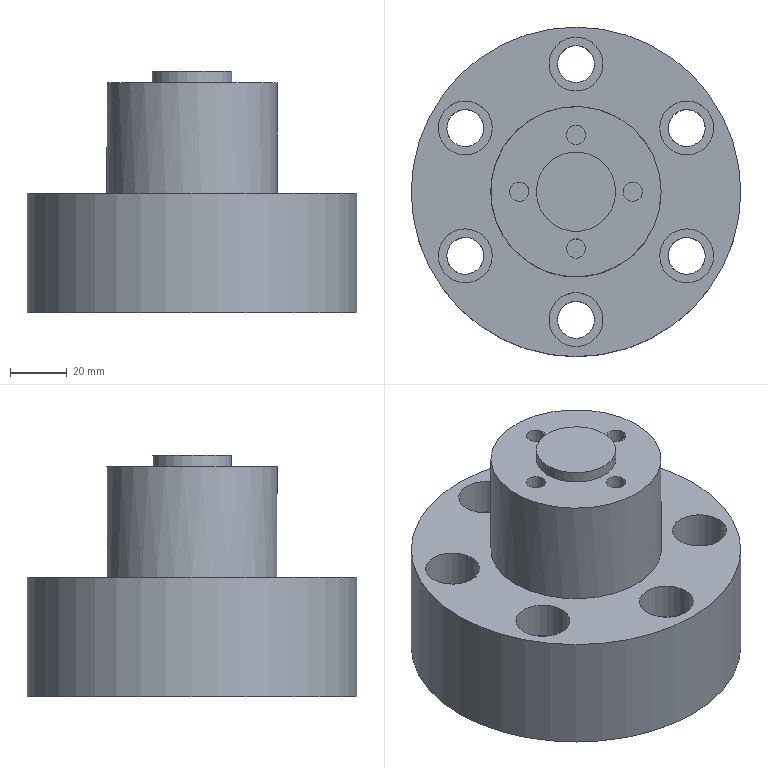Part | NX | 1 solid | 33 faces | box 116 x 116 x 85 mm | volume 509067 mm3 | cylinder 19 | plane 14 | commonest cylinder face diameters 13 x6 19 x6 6.8 x4 28 x1 60 x1 116 x1
STEP:
#1=CARTESIAN_POINT('',(-42.221,16.871,-85.));
#2=VERTEX_POINT('',#1);
#3=CARTESIAN_POINT('',(-38.971,22.5,-85.));
#4=DIRECTION('',(0.,0.,1.));
#5=DIRECTION('',(-0.5,-0.866,0.));
#6=AXIS2_PLACEMENT_3D('',#3,#4,#5);
#7=CIRCLE('',#6,6.5);
#8=EDGE_CURVE('',#2,#2,#7,.T.);
#9=ORIENTED_EDGE('',*,*,#8,.F.);
#10=EDGE_LOOP('',(#9));
#11=FACE_BOUND('',#10,.T.);
#12=CARTESIAN_POINT('',(-32.471,22.5,-56.));
#13=VERTEX_POINT('',#12);
#14=CARTESIAN_POINT('',(-38.971,22.5,-56.));
#15=DIRECTION('',(0.,0.,1.));
#16=DIRECTION('',(1.,0.,0.));
#17=AXIS2_PLACEMENT_3D('',#14,#15,#16);
#18=CIRCLE('',#17,6.5);
#19=EDGE_CURVE('',#13,#13,#18,.F.);
#20=ORIENTED_EDGE('',*,*,#19,.F.);
#21=EDGE_LOOP('',(#20));
#22=FACE_BOUND('',#21,.T.);
#23=CARTESIAN_POINT('',(-38.971,22.5,-85.));
#24=DIRECTION('',(0.,0.,1.));
#25=DIRECTION('',(1.,0.,0.));
#26=AXIS2_PLACEMENT_3D('',#23,#24,#25);
#27=CYLINDRICAL_SURFACE('',#26,6.5);
#28=ADVANCED_FACE('',(#11,#22),#27,.F.);
#29=CARTESIAN_POINT('',(6.5,-45.,-85.));
#30=VERTEX_POINT('',#29);
#31=CARTESIAN_POINT('',(0.,-45.,-85.));
#32=DIRECTION('',(0.,0.,1.));
#33=DIRECTION('',(1.,0.,0.));
#34=AXIS2_PLACEMENT_3D('',#31,#32,#33);
#35=CIRCLE('',#34,6.5);
#36=EDGE_CURVE('',#30,#30,#35,.T.);
#37=ORIENTED_EDGE('',*,*,#36,.F.);
#38=EDGE_LOOP('',(#37));
#39=FACE_BOUND('',#38,.T.);
#40=CARTESIAN_POINT('',(6.5,-45.,-56.));
#41=VERTEX_POINT('',#40);
#42=CARTESIAN_POINT('',(0.,-45.,-56.));
#43=DIRECTION('',(0.,0.,1.));
#44=DIRECTION('',(1.,0.,0.));
#45=AXIS2_PLACEMENT_3D('',#42,#43,#44);
#46=CIRCLE('',#45,6.5);
#47=EDGE_CURVE('',#41,#41,#46,.F.);
#48=ORIENTED_EDGE('',*,*,#47,.F.);
#49=EDGE_LOOP('',(#48));
#50=FACE_BOUND('',#49,.T.);
#51=CARTESIAN_POINT('',(0.,-45.,-85.));
#52=DIRECTION('',(0.,0.,1.));
#53=DIRECTION('',(1.,0.,0.));
#54=AXIS2_PLACEMENT_3D('',#51,#52,#53);
#55=CYLINDRICAL_SURFACE('',#54,6.5);
#56=ADVANCED_FACE('',(#39,#50),#55,.F.);
#57=CARTESIAN_POINT('',(-6.5,45.,-85.));
#58=VERTEX_POINT('',#57);
#59=CARTESIAN_POINT('',(0.,45.,-85.));
#60=DIRECTION('',(0.,0.,1.));
#61=DIRECTION('',(-1.,0.,0.));
#62=AXIS2_PLACEMENT_3D('',#59,#60,#61);
#63=CIRCLE('',#62,6.5);
#64=EDGE_CURVE('',#58,#58,#63,.T.);
#65=ORIENTED_EDGE('',*,*,#64,.F.);
#66=EDGE_LOOP('',(#65));
#67=FACE_BOUND('',#66,.T.);
#68=CARTESIAN_POINT('',(6.5,45.,-56.));
#69=VERTEX_POINT('',#68);
#70=CARTESIAN_POINT('',(0.,45.,-56.));
#71=DIRECTION('',(0.,0.,1.));
#72=DIRECTION('',(1.,0.,0.));
#73=AXIS2_PLACEMENT_3D('',#70,#71,#72);
#74=CIRCLE('',#73,6.5);
#75=EDGE_CURVE('',#69,#69,#74,.F.);
#76=ORIENTED_EDGE('',*,*,#75,.F.);
#77=EDGE_LOOP('',(#76));
#78=FACE_BOUND('',#77,.T.);
#79=CARTESIAN_POINT('',(0.,45.,-85.));
#80=DIRECTION('',(0.,0.,1.));
#81=DIRECTION('',(1.,0.,0.));
#82=AXIS2_PLACEMENT_3D('',#79,#80,#81);
#83=CYLINDRICAL_SURFACE('',#82,6.5);
#84=ADVANCED_FACE('',(#67,#78),#83,.F.);
#85=CARTESIAN_POINT('',(42.221,-16.871,-85.));
#86=VERTEX_POINT('',#85);
#87=CARTESIAN_POINT('',(38.971,-22.5,-85.));
#88=DIRECTION('',(0.,0.,1.));
#89=DIRECTION('',(0.5,0.866,0.));
#90=AXIS2_PLACEMENT_3D('',#87,#88,#89);
#91=CIRCLE('',#90,6.5);
#92=EDGE_CURVE('',#86,#86,#91,.T.);
#93=ORIENTED_EDGE('',*,*,#92,.F.);
#94=EDGE_LOOP('',(#93));
#95=FACE_BOUND('',#94,.T.);
#96=CARTESIAN_POINT('',(45.471,-22.5,-56.));
#97=VERTEX_POINT('',#96);
#98=CARTESIAN_POINT('',(38.971,-22.5,-56.));
#99=DIRECTION('',(0.,0.,1.));
#100=DIRECTION('',(1.,0.,0.));
#101=AXIS2_PLACEMENT_3D('',#98,#99,#100);
#102=CIRCLE('',#101,6.5);
#103=EDGE_CURVE('',#97,#97,#102,.F.);
#104=ORIENTED_EDGE('',*,*,#103,.F.);
#105=EDGE_LOOP('',(#104));
#106=FACE_BOUND('',#105,.T.);
#107=CARTESIAN_POINT('',(38.971,-22.5,-85.));
#108=DIRECTION('',(0.,0.,1.));
#109=DIRECTION('',(1.,0.,0.));
#110=AXIS2_PLACEMENT_3D('',#107,#108,#109);
#111=CYLINDRICAL_SURFACE('',#110,6.5);
#112=ADVANCED_FACE('',(#95,#106),#111,.F.);
#113=CARTESIAN_POINT('',(35.721,28.129,-85.));
#114=VERTEX_POINT('',#113);
#115=CARTESIAN_POINT('',(38.971,22.5,-85.));
#116=DIRECTION('',(0.,0.,1.));
#117=DIRECTION('',(-0.5,0.866,0.));
#118=AXIS2_PLACEMENT_3D('',#115,#116,#117);
#119=CIRCLE('',#118,6.5);
#120=EDGE_CURVE('',#114,#114,#119,.T.);
#121=ORIENTED_EDGE('',*,*,#120,.F.);
#122=EDGE_LOOP('',(#121));
#123=FACE_BOUND('',#122,.T.);
#124=CARTESIAN_POINT('',(45.471,22.5,-56.));
#125=VERTEX_POINT('',#124);
#126=CARTESIAN_POINT('',(38.971,22.5,-56.));
#127=DIRECTION('',(0.,0.,1.));
#128=DIRECTION('',(1.,0.,0.));
#129=AXIS2_PLACEMENT_3D('',#126,#127,#128);
#130=CIRCLE('',#129,6.5);
#131=EDGE_CURVE('',#125,#125,#130,.F.);
#132=ORIENTED_EDGE('',*,*,#131,.F.);
#133=EDGE_LOOP('',(#132));
#134=FACE_BOUND('',#133,.T.);
#135=CARTESIAN_POINT('',(38.971,22.5,-85.));
#136=DIRECTION('',(0.,0.,1.));
#137=DIRECTION('',(1.,0.,0.));
#138=AXIS2_PLACEMENT_3D('',#135,#136,#137);
#139=CYLINDRICAL_SURFACE('',#138,6.5);
#140=ADVANCED_FACE('',(#123,#134),#139,.F.);
#141=CARTESIAN_POINT('',(-43.721,14.273,-43.));
#142=VERTEX_POINT('',#141);
#143=CARTESIAN_POINT('',(-38.971,22.5,-43.));
#144=DIRECTION('',(0.,0.,1.));
#145=DIRECTION('',(-0.5,-0.866,0.));
#146=AXIS2_PLACEMENT_3D('',#143,#144,#145);
#147=CIRCLE('',#146,9.5);
#148=EDGE_CURVE('',#142,#142,#147,.T.);
#149=ORIENTED_EDGE('',*,*,#148,.F.);
#150=EDGE_LOOP('',(#149));
#151=FACE_BOUND('',#150,.T.);
#152=CARTESIAN_POINT('',(9.5,-45.,-43.));
#153=VERTEX_POINT('',#152);
#154=CARTESIAN_POINT('',(0.,-45.,-43.));
#155=DIRECTION('',(0.,0.,1.));
#156=DIRECTION('',(1.,0.,0.));
#157=AXIS2_PLACEMENT_3D('',#154,#155,#156);
#158=CIRCLE('',#157,9.5);
#159=EDGE_CURVE('',#153,#153,#158,.T.);
#160=ORIENTED_EDGE('',*,*,#159,.F.);
#161=EDGE_LOOP('',(#160));
#162=FACE_BOUND('',#161,.T.);
#163=CARTESIAN_POINT('',(-9.5,45.,-43.));
#164=VERTEX_POINT('',#163);
#165=CARTESIAN_POINT('',(0.,45.,-43.));
#166=DIRECTION('',(0.,0.,1.));
#167=DIRECTION('',(-1.,0.,0.));
#168=AXIS2_PLACEMENT_3D('',#165,#166,#167);
#169=CIRCLE('',#168,9.5);
#170=EDGE_CURVE('',#164,#164,#169,.T.);
#171=ORIENTED_EDGE('',*,*,#170,.F.);
#172=EDGE_LOOP('',(#171));
#173=FACE_BOUND('',#172,.T.);
#174=CARTESIAN_POINT('',(43.721,-14.273,-43.));
#175=VERTEX_POINT('',#174);
#176=CARTESIAN_POINT('',(38.971,-22.5,-43.));
#177=DIRECTION('',(0.,0.,1.));
#178=DIRECTION('',(0.5,0.866,0.));
#179=AXIS2_PLACEMENT_3D('',#176,#177,#178);
#180=CIRCLE('',#179,9.5);
#181=EDGE_CURVE('',#175,#175,#180,.T.);
#182=ORIENTED_EDGE('',*,*,#181,.F.);
#183=EDGE_LOOP('',(#182));
#184=FACE_BOUND('',#183,.T.);
#185=CARTESIAN_POINT('',(58.,0.,-43.));
#186=VERTEX_POINT('',#185);
#187=CARTESIAN_POINT('',(0.,0.,-43.));
#188=DIRECTION('',(0.,0.,-1.));
#189=DIRECTION('',(1.,0.,0.));
#190=AXIS2_PLACEMENT_3D('',#187,#188,#189);
#191=CIRCLE('',#190,58.);
#192=EDGE_CURVE('',#186,#186,#191,.T.);
#193=ORIENTED_EDGE('',*,*,#192,.F.);
#194=EDGE_LOOP('',(#193));
#195=FACE_BOUND('',#194,.T.);
#196=CARTESIAN_POINT('',(-30.,0.,-43.));
#197=VERTEX_POINT('',#196);
#198=CARTESIAN_POINT('',(0.,0.,-43.));
#199=DIRECTION('',(0.,0.,-1.));
#200=DIRECTION('',(-1.,0.,0.));
#201=AXIS2_PLACEMENT_3D('',#198,#199,#200);
#202=CIRCLE('',#201,30.);
#203=EDGE_CURVE('',#197,#197,#202,.T.);
#204=ORIENTED_EDGE('',*,*,#203,.T.);
#205=EDGE_LOOP('',(#204));
#206=FACE_BOUND('',#205,.T.);
#207=CARTESIAN_POINT('',(34.221,30.727,-43.));
#208=VERTEX_POINT('',#207);
#209=CARTESIAN_POINT('',(38.971,22.5,-43.));
#210=DIRECTION('',(0.,0.,1.));
#211=DIRECTION('',(-0.5,0.866,0.));
#212=AXIS2_PLACEMENT_3D('',#209,#210,#211);
#213=CIRCLE('',#212,9.5);
#214=EDGE_CURVE('',#208,#208,#213,.T.);
#215=ORIENTED_EDGE('',*,*,#214,.F.);
#216=EDGE_LOOP('',(#215));
#217=FACE_BOUND('',#216,.T.);
#218=CARTESIAN_POINT('',(-34.221,-30.727,-43.));
#219=VERTEX_POINT('',#218);
#220=CARTESIAN_POINT('',(-38.971,-22.5,-43.));
#221=DIRECTION('',(0.,0.,-1.));
#222=DIRECTION('',(0.5,-0.866,0.));
#223=AXIS2_PLACEMENT_3D('',#220,#221,#222);
#224=CIRCLE('',#223,9.5);
#225=EDGE_CURVE('',#219,#219,#224,.T.);
#226=ORIENTED_EDGE('',*,*,#225,.T.);
#227=EDGE_LOOP('',(#226));
#228=FACE_BOUND('',#227,.T.);
#229=CARTESIAN_POINT('',(19.486,11.25,-43.));
#230=DIRECTION('',(0.,0.,-1.));
#231=DIRECTION('',(-1.,0.,0.));
#232=AXIS2_PLACEMENT_3D('',#229,#230,#231);
#233=PLANE('',#232);
#234=ADVANCED_FACE('',(#151,#162,#173,#184,#195,#206,#217,#228),#233,.F.);
#235=CARTESIAN_POINT('',(30.,0.,-4.));
#236=VERTEX_POINT('',#235);
#237=CARTESIAN_POINT('',(0.,0.,-4.));
#238=DIRECTION('',(0.,0.,-1.));
#239=DIRECTION('',(1.,0.,0.));
#240=AXIS2_PLACEMENT_3D('',#237,#238,#239);
#241=CIRCLE('',#240,30.);
#242=EDGE_CURVE('',#236,#236,#241,.T.);
#243=ORIENTED_EDGE('',*,*,#242,.T.);
#244=EDGE_LOOP('',(#243));
#245=FACE_BOUND('',#244,.T.);
#246=ORIENTED_EDGE('',*,*,#203,.F.);
#247=EDGE_LOOP('',(#246));
#248=FACE_BOUND('',#247,.T.);
#249=CARTESIAN_POINT('',(0.,0.,-85.));
#250=DIRECTION('',(0.,0.,1.));
#251=DIRECTION('',(1.,0.,0.));
#252=AXIS2_PLACEMENT_3D('',#249,#250,#251);
#253=CYLINDRICAL_SURFACE('',#252,30.);
#254=ADVANCED_FACE('',(#245,#248),#253,.T.);
#255=CARTESIAN_POINT('',(-3.4,20.,-4.));
#256=VERTEX_POINT('',#255);
#257=CARTESIAN_POINT('',(0.,20.,-4.));
#258=DIRECTION('',(0.,0.,-1.));
#259=DIRECTION('',(-1.,0.,0.));
#260=AXIS2_PLACEMENT_3D('',#257,#258,#259);
#261=CIRCLE('',#260,3.4);
#262=EDGE_CURVE('',#256,#256,#261,.T.);
#263=ORIENTED_EDGE('',*,*,#262,.T.);
#264=EDGE_LOOP('',(#263));
#265=FACE_BOUND('',#264,.T.);
#266=ORIENTED_EDGE('',*,*,#242,.F.);
#267=EDGE_LOOP('',(#266));
#268=FACE_BOUND('',#267,.T.);
#269=CARTESIAN_POINT('',(-14.,0.,-4.));
#270=VERTEX_POINT('',#269);
#271=CARTESIAN_POINT('',(0.,0.,-4.));
#272=DIRECTION('',(0.,0.,-1.));
#273=DIRECTION('',(-1.,0.,0.));
#274=AXIS2_PLACEMENT_3D('',#271,#272,#273);
#275=CIRCLE('',#274,14.);
#276=EDGE_CURVE('',#270,#270,#275,.F.);
#277=ORIENTED_EDGE('',*,*,#276,.F.);
#278=EDGE_LOOP('',(#277));
#279=FACE_BOUND('',#278,.T.);
#280=CARTESIAN_POINT('',(-23.4,0.,-4.));
#281=VERTEX_POINT('',#280);
#282=CARTESIAN_POINT('',(-20.,0.,-4.));
#283=DIRECTION('',(0.,0.,-1.));
#284=DIRECTION('',(-1.,0.,0.));
#285=AXIS2_PLACEMENT_3D('',#282,#283,#284);
#286=CIRCLE('',#285,3.4);
#287=EDGE_CURVE('',#281,#281,#286,.F.);
#288=ORIENTED_EDGE('',*,*,#287,.F.);
#289=EDGE_LOOP('',(#288));
#290=FACE_BOUND('',#289,.T.);
#291=CARTESIAN_POINT('',(-3.4,-20.,-4.));
#292=VERTEX_POINT('',#291);
#293=CARTESIAN_POINT('',(0.,-20.,-4.));
#294=DIRECTION('',(0.,0.,-1.));
#295=DIRECTION('',(-1.,0.,0.));
#296=AXIS2_PLACEMENT_3D('',#293,#294,#295);
#297=CIRCLE('',#296,3.4);
#298=EDGE_CURVE('',#292,#292,#297,.T.);
#299=ORIENTED_EDGE('',*,*,#298,.T.);
#300=EDGE_LOOP('',(#299));
#301=FACE_BOUND('',#300,.T.);
#302=CARTESIAN_POINT('',(16.6,0.,-4.));
#303=VERTEX_POINT('',#302);
#304=CARTESIAN_POINT('',(20.,0.,-4.));
#305=DIRECTION('',(0.,0.,-1.));
#306=DIRECTION('',(-1.,0.,0.));
#307=AXIS2_PLACEMENT_3D('',#304,#305,#306);
#308=CIRCLE('',#307,3.4);
#309=EDGE_CURVE('',#303,#303,#308,.T.);
#310=ORIENTED_EDGE('',*,*,#309,.T.);
#311=EDGE_LOOP('',(#310));
#312=FACE_BOUND('',#311,.T.);
#313=CARTESIAN_POINT('',(0.,0.,-4.));
#314=DIRECTION('',(0.,0.,-1.));
#315=DIRECTION('',(-1.,0.,0.));
#316=AXIS2_PLACEMENT_3D('',#313,#314,#315);
#317=PLANE('',#316);
#318=ADVANCED_FACE('',(#265,#268,#279,#290,#301,#312),#317,.F.);
#319=CARTESIAN_POINT('',(14.,0.,0.));
#320=VERTEX_POINT('',#319);
#321=CARTESIAN_POINT('',(0.,0.,0.));
#322=DIRECTION('',(0.,0.,1.));
#323=DIRECTION('',(1.,0.,0.));
#324=AXIS2_PLACEMENT_3D('',#321,#322,#323);
#325=CIRCLE('',#324,14.);
#326=EDGE_CURVE('',#320,#320,#325,.T.);
#327=ORIENTED_EDGE('',*,*,#326,.F.);
#328=EDGE_LOOP('',(#327));
#329=FACE_BOUND('',#328,.T.);
#330=ORIENTED_EDGE('',*,*,#276,.T.);
#331=EDGE_LOOP('',(#330));
#332=FACE_BOUND('',#331,.T.);
#333=CARTESIAN_POINT('',(0.,0.,-85.));
#334=DIRECTION('',(0.,0.,1.));
#335=DIRECTION('',(1.,0.,0.));
#336=AXIS2_PLACEMENT_3D('',#333,#334,#335);
#337=CYLINDRICAL_SURFACE('',#336,14.);
#338=ADVANCED_FACE('',(#329,#332),#337,.T.);
#339=ORIENTED_EDGE('',*,*,#326,.T.);
#340=EDGE_LOOP('',(#339));
#341=FACE_BOUND('',#340,.T.);
#342=CARTESIAN_POINT('',(0.,0.,0.));
#343=DIRECTION('',(0.,0.,1.));
#344=DIRECTION('',(1.,0.,0.));
#345=AXIS2_PLACEMENT_3D('',#342,#343,#344);
#346=PLANE('',#345);
#347=ADVANCED_FACE('',(#341),#346,.T.);
#348=CARTESIAN_POINT('',(-20.,-3.4,-20.));
#349=VERTEX_POINT('',#348);
#350=CARTESIAN_POINT('',(-20.,0.,-20.));
#351=DIRECTION('',(0.,0.,-1.));
#352=DIRECTION('',(0.,-1.,0.));
#353=AXIS2_PLACEMENT_3D('',#350,#351,#352);
#354=CIRCLE('',#353,3.4);
#355=EDGE_CURVE('',#349,#349,#354,.F.);
#356=ORIENTED_EDGE('',*,*,#355,.F.);
#357=EDGE_LOOP('',(#356));
#358=FACE_BOUND('',#357,.T.);
#359=ORIENTED_EDGE('',*,*,#287,.T.);
#360=EDGE_LOOP('',(#359));
#361=FACE_BOUND('',#360,.T.);
#362=CARTESIAN_POINT('',(-20.,0.,-20.));
#363=DIRECTION('',(0.,0.,1.));
#364=DIRECTION('',(1.,0.,0.));
#365=AXIS2_PLACEMENT_3D('',#362,#363,#364);
#366=CYLINDRICAL_SURFACE('',#365,3.4);
#367=ADVANCED_FACE('',(#358,#361),#366,.F.);
#368=ORIENTED_EDGE('',*,*,#355,.T.);
#369=EDGE_LOOP('',(#368));
#370=FACE_BOUND('',#369,.T.);
#371=CARTESIAN_POINT('',(-20.,0.,-20.));
#372=DIRECTION('',(0.,0.,-1.));
#373=DIRECTION('',(-1.,0.,0.));
#374=AXIS2_PLACEMENT_3D('',#371,#372,#373);
#375=PLANE('',#374);
#376=ADVANCED_FACE('',(#370),#375,.F.);
#377=CARTESIAN_POINT('',(3.4,-20.,-20.));
#378=VERTEX_POINT('',#377);
#379=CARTESIAN_POINT('',(0.,-20.,-20.));
#380=DIRECTION('',(0.,0.,1.));
#381=DIRECTION('',(1.,0.,0.));
#382=AXIS2_PLACEMENT_3D('',#379,#380,#381);
#383=CIRCLE('',#382,3.4);
#384=EDGE_CURVE('',#378,#378,#383,.F.);
#385=ORIENTED_EDGE('',*,*,#384,.T.);
#386=EDGE_LOOP('',(#385));
#387=FACE_BOUND('',#386,.T.);
#388=ORIENTED_EDGE('',*,*,#298,.F.);
#389=EDGE_LOOP('',(#388));
#390=FACE_BOUND('',#389,.T.);
#391=CARTESIAN_POINT('',(0.,-20.,-20.));
#392=DIRECTION('',(0.,0.,1.));
#393=DIRECTION('',(1.,0.,0.));
#394=AXIS2_PLACEMENT_3D('',#391,#392,#393);
#395=CYLINDRICAL_SURFACE('',#394,3.4);
#396=ADVANCED_FACE('',(#387,#390),#395,.F.);
#397=ORIENTED_EDGE('',*,*,#384,.F.);
#398=EDGE_LOOP('',(#397));
#399=FACE_BOUND('',#398,.T.);
#400=CARTESIAN_POINT('',(0.,-20.,-20.));
#401=DIRECTION('',(0.,0.,1.));
#402=DIRECTION('',(1.,0.,0.));
#403=AXIS2_PLACEMENT_3D('',#400,#401,#402);
#404=PLANE('',#403);
#405=ADVANCED_FACE('',(#399),#404,.T.);
#406=CARTESIAN_POINT('',(-3.4,20.,-20.));
#407=VERTEX_POINT('',#406);
#408=CARTESIAN_POINT('',(0.,20.,-20.));
#409=DIRECTION('',(0.,0.,1.));
#410=DIRECTION('',(-1.,0.,0.));
#411=AXIS2_PLACEMENT_3D('',#408,#409,#410);
#412=CIRCLE('',#411,3.4);
#413=EDGE_CURVE('',#407,#407,#412,.F.);
#414=ORIENTED_EDGE('',*,*,#413,.T.);
#415=EDGE_LOOP('',(#414));
#416=FACE_BOUND('',#415,.T.);
#417=ORIENTED_EDGE('',*,*,#262,.F.);
#418=EDGE_LOOP('',(#417));
#419=FACE_BOUND('',#418,.T.);
#420=CARTESIAN_POINT('',(0.,20.,-20.));
#421=DIRECTION('',(0.,0.,1.));
#422=DIRECTION('',(1.,0.,0.));
#423=AXIS2_PLACEMENT_3D('',#420,#421,#422);
#424=CYLINDRICAL_SURFACE('',#423,3.4);
#425=ADVANCED_FACE('',(#416,#419),#424,.F.);
#426=ORIENTED_EDGE('',*,*,#413,.F.);
#427=EDGE_LOOP('',(#426));
#428=FACE_BOUND('',#427,.T.);
#429=CARTESIAN_POINT('',(0.,20.,-20.));
#430=DIRECTION('',(0.,0.,1.));
#431=DIRECTION('',(1.,0.,0.));
#432=AXIS2_PLACEMENT_3D('',#429,#430,#431);
#433=PLANE('',#432);
#434=ADVANCED_FACE('',(#428),#433,.T.);
#435=CARTESIAN_POINT('',(20.,3.4,-20.));
#436=VERTEX_POINT('',#435);
#437=CARTESIAN_POINT('',(20.,0.,-20.));
#438=DIRECTION('',(0.,0.,1.));
#439=DIRECTION('',(0.,1.,0.));
#440=AXIS2_PLACEMENT_3D('',#437,#438,#439);
#441=CIRCLE('',#440,3.4);
#442=EDGE_CURVE('',#436,#436,#441,.F.);
#443=ORIENTED_EDGE('',*,*,#442,.T.);
#444=EDGE_LOOP('',(#443));
#445=FACE_BOUND('',#444,.T.);
#446=ORIENTED_EDGE('',*,*,#309,.F.);
#447=EDGE_LOOP('',(#446));
#448=FACE_BOUND('',#447,.T.);
#449=CARTESIAN_POINT('',(20.,0.,-20.));
#450=DIRECTION('',(0.,0.,1.));
#451=DIRECTION('',(1.,0.,0.));
#452=AXIS2_PLACEMENT_3D('',#449,#450,#451);
#453=CYLINDRICAL_SURFACE('',#452,3.4);
#454=ADVANCED_FACE('',(#445,#448),#453,.F.);
#455=ORIENTED_EDGE('',*,*,#442,.F.);
#456=EDGE_LOOP('',(#455));
#457=FACE_BOUND('',#456,.T.);
#458=CARTESIAN_POINT('',(20.,0.,-20.));
#459=DIRECTION('',(0.,0.,1.));
#460=DIRECTION('',(1.,0.,0.));
#461=AXIS2_PLACEMENT_3D('',#458,#459,#460);
#462=PLANE('',#461);
#463=ADVANCED_FACE('',(#457),#462,.T.);
#464=CARTESIAN_POINT('',(58.,0.,-85.));
#465=VERTEX_POINT('',#464);
#466=CARTESIAN_POINT('',(0.,0.,-85.));
#467=DIRECTION('',(0.,0.,-1.));
#468=DIRECTION('',(1.,0.,0.));
#469=AXIS2_PLACEMENT_3D('',#466,#467,#468);
#470=CIRCLE('',#469,58.);
#471=EDGE_CURVE('',#465,#465,#470,.T.);
#472=ORIENTED_EDGE('',*,*,#471,.F.);
#473=EDGE_LOOP('',(#472));
#474=FACE_BOUND('',#473,.T.);
#475=ORIENTED_EDGE('',*,*,#192,.T.);
#476=EDGE_LOOP('',(#475));
#477=FACE_BOUND('',#476,.T.);
#478=CARTESIAN_POINT('',(0.,0.,-85.));
#479=DIRECTION('',(0.,0.,1.));
#480=DIRECTION('',(1.,0.,0.));
#481=AXIS2_PLACEMENT_3D('',#478,#479,#480);
#482=CYLINDRICAL_SURFACE('',#481,58.);
#483=ADVANCED_FACE('',(#474,#477),#482,.T.);
#484=CARTESIAN_POINT('',(-45.471,-22.5,-56.));
#485=VERTEX_POINT('',#484);
#486=CARTESIAN_POINT('',(-38.971,-22.5,-56.));
#487=DIRECTION('',(0.,0.,-1.));
#488=DIRECTION('',(-1.,0.,0.));
#489=AXIS2_PLACEMENT_3D('',#486,#487,#488);
#490=CIRCLE('',#489,6.5);
#491=EDGE_CURVE('',#485,#485,#490,.F.);
#492=ORIENTED_EDGE('',*,*,#491,.T.);
#493=EDGE_LOOP('',(#492));
#494=FACE_BOUND('',#493,.T.);
#495=CARTESIAN_POINT('',(-35.721,-28.129,-85.));
#496=VERTEX_POINT('',#495);
#497=CARTESIAN_POINT('',(-38.971,-22.5,-85.));
#498=DIRECTION('',(0.,0.,1.));
#499=DIRECTION('',(0.5,-0.866,0.));
#500=AXIS2_PLACEMENT_3D('',#497,#498,#499);
#501=CIRCLE('',#500,6.5);
#502=EDGE_CURVE('',#496,#496,#501,.T.);
#503=ORIENTED_EDGE('',*,*,#502,.F.);
#504=EDGE_LOOP('',(#503));
#505=FACE_BOUND('',#504,.T.);
#506=CARTESIAN_POINT('',(-38.971,-22.5,-85.));
#507=DIRECTION('',(0.,0.,1.));
#508=DIRECTION('',(1.,0.,0.));
#509=AXIS2_PLACEMENT_3D('',#506,#507,#508);
#510=CYLINDRICAL_SURFACE('',#509,6.5);
#511=ADVANCED_FACE('',(#494,#505),#510,.F.);
#512=ORIENTED_EDGE('',*,*,#471,.T.);
#513=EDGE_LOOP('',(#512));
#514=FACE_BOUND('',#513,.T.);
#515=ORIENTED_EDGE('',*,*,#120,.T.);
#516=EDGE_LOOP('',(#515));
#517=FACE_BOUND('',#516,.T.);
#518=ORIENTED_EDGE('',*,*,#92,.T.);
#519=EDGE_LOOP('',(#518));
#520=FACE_BOUND('',#519,.T.);
#521=ORIENTED_EDGE('',*,*,#64,.T.);
#522=EDGE_LOOP('',(#521));
#523=FACE_BOUND('',#522,.T.);
#524=ORIENTED_EDGE('',*,*,#36,.T.);
#525=EDGE_LOOP('',(#524));
#526=FACE_BOUND('',#525,.T.);
#527=ORIENTED_EDGE('',*,*,#8,.T.);
#528=EDGE_LOOP('',(#527));
#529=FACE_BOUND('',#528,.T.);
#530=ORIENTED_EDGE('',*,*,#502,.T.);
#531=EDGE_LOOP('',(#530));
#532=FACE_BOUND('',#531,.T.);
#533=CARTESIAN_POINT('',(0.,0.,-85.));
#534=DIRECTION('',(0.,0.,1.));
#535=DIRECTION('',(1.,0.,0.));
#536=AXIS2_PLACEMENT_3D('',#533,#534,#535);
#537=PLANE('',#536);
#538=ADVANCED_FACE('',(#514,#517,#520,#523,#526,#529,#532),#537,.F.);
#539=CARTESIAN_POINT('',(34.221,30.727,-56.));
#540=VERTEX_POINT('',#539);
#541=CARTESIAN_POINT('',(38.971,22.5,-56.));
#542=DIRECTION('',(0.,0.,1.));
#543=DIRECTION('',(-0.5,0.866,0.));
#544=AXIS2_PLACEMENT_3D('',#541,#542,#543);
#545=CIRCLE('',#544,9.5);
#546=EDGE_CURVE('',#540,#540,#545,.F.);
#547=ORIENTED_EDGE('',*,*,#546,.F.);
#548=EDGE_LOOP('',(#547));
#549=FACE_BOUND('',#548,.T.);
#550=ORIENTED_EDGE('',*,*,#131,.T.);
#551=EDGE_LOOP('',(#550));
#552=FACE_BOUND('',#551,.T.);
#553=CARTESIAN_POINT('',(38.971,22.5,-56.));
#554=DIRECTION('',(0.,0.,1.));
#555=DIRECTION('',(1.,0.,0.));
#556=AXIS2_PLACEMENT_3D('',#553,#554,#555);
#557=PLANE('',#556);
#558=ADVANCED_FACE('',(#549,#552),#557,.T.);
#559=ORIENTED_EDGE('',*,*,#546,.T.);
#560=EDGE_LOOP('',(#559));
#561=FACE_BOUND('',#560,.T.);
#562=ORIENTED_EDGE('',*,*,#214,.T.);
#563=EDGE_LOOP('',(#562));
#564=FACE_BOUND('',#563,.T.);
#565=CARTESIAN_POINT('',(38.971,22.5,-56.));
#566=DIRECTION('',(0.,0.,1.));
#567=DIRECTION('',(1.,0.,0.));
#568=AXIS2_PLACEMENT_3D('',#565,#566,#567);
#569=CYLINDRICAL_SURFACE('',#568,9.5);
#570=ADVANCED_FACE('',(#561,#564),#569,.F.);
#571=CARTESIAN_POINT('',(-34.221,-30.727,-56.));
#572=VERTEX_POINT('',#571);
#573=CARTESIAN_POINT('',(-38.971,-22.5,-56.));
#574=DIRECTION('',(0.,0.,-1.));
#575=DIRECTION('',(0.5,-0.866,0.));
#576=AXIS2_PLACEMENT_3D('',#573,#574,#575);
#577=CIRCLE('',#576,9.5);
#578=EDGE_CURVE('',#572,#572,#577,.F.);
#579=ORIENTED_EDGE('',*,*,#578,.T.);
#580=EDGE_LOOP('',(#579));
#581=FACE_BOUND('',#580,.T.);
#582=ORIENTED_EDGE('',*,*,#491,.F.);
#583=EDGE_LOOP('',(#582));
#584=FACE_BOUND('',#583,.T.);
#585=CARTESIAN_POINT('',(-38.971,-22.5,-56.));
#586=DIRECTION('',(0.,0.,-1.));
#587=DIRECTION('',(-1.,0.,0.));
#588=AXIS2_PLACEMENT_3D('',#585,#586,#587);
#589=PLANE('',#588);
#590=ADVANCED_FACE('',(#581,#584),#589,.F.);
#591=ORIENTED_EDGE('',*,*,#578,.F.);
#592=EDGE_LOOP('',(#591));
#593=FACE_BOUND('',#592,.T.);
#594=ORIENTED_EDGE('',*,*,#225,.F.);
#595=EDGE_LOOP('',(#594));
#596=FACE_BOUND('',#595,.T.);
#597=CARTESIAN_POINT('',(-38.971,-22.5,-56.));
#598=DIRECTION('',(0.,0.,1.));
#599=DIRECTION('',(1.,0.,0.));
#600=AXIS2_PLACEMENT_3D('',#597,#598,#599);
#601=CYLINDRICAL_SURFACE('',#600,9.5);
#602=ADVANCED_FACE('',(#593,#596),#601,.F.);
#603=CARTESIAN_POINT('',(43.721,-14.273,-56.));
#604=VERTEX_POINT('',#603);
#605=CARTESIAN_POINT('',(38.971,-22.5,-56.));
#606=DIRECTION('',(0.,0.,1.));
#607=DIRECTION('',(0.5,0.866,0.));
#608=AXIS2_PLACEMENT_3D('',#605,#606,#607);
#609=CIRCLE('',#608,9.5);
#610=EDGE_CURVE('',#604,#604,#609,.F.);
#611=ORIENTED_EDGE('',*,*,#610,.F.);
#612=EDGE_LOOP('',(#611));
#613=FACE_BOUND('',#612,.T.);
#614=ORIENTED_EDGE('',*,*,#103,.T.);
#615=EDGE_LOOP('',(#614));
#616=FACE_BOUND('',#615,.T.);
#617=CARTESIAN_POINT('',(38.971,-22.5,-56.));
#618=DIRECTION('',(0.,0.,1.));
#619=DIRECTION('',(1.,0.,0.));
#620=AXIS2_PLACEMENT_3D('',#617,#618,#619);
#621=PLANE('',#620);
#622=ADVANCED_FACE('',(#613,#616),#621,.T.);
#623=ORIENTED_EDGE('',*,*,#610,.T.);
#624=EDGE_LOOP('',(#623));
#625=FACE_BOUND('',#624,.T.);
#626=ORIENTED_EDGE('',*,*,#181,.T.);
#627=EDGE_LOOP('',(#626));
#628=FACE_BOUND('',#627,.T.);
#629=CARTESIAN_POINT('',(38.971,-22.5,-56.));
#630=DIRECTION('',(0.,0.,1.));
#631=DIRECTION('',(1.,0.,0.));
#632=AXIS2_PLACEMENT_3D('',#629,#630,#631);
#633=CYLINDRICAL_SURFACE('',#632,9.5);
#634=ADVANCED_FACE('',(#625,#628),#633,.F.);
#635=CARTESIAN_POINT('',(-9.5,45.,-56.));
#636=VERTEX_POINT('',#635);
#637=CARTESIAN_POINT('',(0.,45.,-56.));
#638=DIRECTION('',(0.,0.,1.));
#639=DIRECTION('',(-1.,0.,0.));
#640=AXIS2_PLACEMENT_3D('',#637,#638,#639);
#641=CIRCLE('',#640,9.5);
#642=EDGE_CURVE('',#636,#636,#641,.F.);
#643=ORIENTED_EDGE('',*,*,#642,.F.);
#644=EDGE_LOOP('',(#643));
#645=FACE_BOUND('',#644,.T.);
#646=ORIENTED_EDGE('',*,*,#75,.T.);
#647=EDGE_LOOP('',(#646));
#648=FACE_BOUND('',#647,.T.);
#649=CARTESIAN_POINT('',(0.,45.,-56.));
#650=DIRECTION('',(0.,0.,1.));
#651=DIRECTION('',(1.,0.,0.));
#652=AXIS2_PLACEMENT_3D('',#649,#650,#651);
#653=PLANE('',#652);
#654=ADVANCED_FACE('',(#645,#648),#653,.T.);
#655=ORIENTED_EDGE('',*,*,#642,.T.);
#656=EDGE_LOOP('',(#655));
#657=FACE_BOUND('',#656,.T.);
#658=ORIENTED_EDGE('',*,*,#170,.T.);
#659=EDGE_LOOP('',(#658));
#660=FACE_BOUND('',#659,.T.);
#661=CARTESIAN_POINT('',(0.,45.,-56.));
#662=DIRECTION('',(0.,0.,1.));
#663=DIRECTION('',(1.,0.,0.));
#664=AXIS2_PLACEMENT_3D('',#661,#662,#663);
#665=CYLINDRICAL_SURFACE('',#664,9.5);
#666=ADVANCED_FACE('',(#657,#660),#665,.F.);
#667=CARTESIAN_POINT('',(9.5,-45.,-56.));
#668=VERTEX_POINT('',#667);
#669=CARTESIAN_POINT('',(0.,-45.,-56.));
#670=DIRECTION('',(0.,0.,1.));
#671=DIRECTION('',(1.,0.,0.));
#672=AXIS2_PLACEMENT_3D('',#669,#670,#671);
#673=CIRCLE('',#672,9.5);
#674=EDGE_CURVE('',#668,#668,#673,.F.);
#675=ORIENTED_EDGE('',*,*,#674,.F.);
#676=EDGE_LOOP('',(#675));
#677=FACE_BOUND('',#676,.T.);
#678=ORIENTED_EDGE('',*,*,#47,.T.);
#679=EDGE_LOOP('',(#678));
#680=FACE_BOUND('',#679,.T.);
#681=CARTESIAN_POINT('',(0.,-45.,-56.));
#682=DIRECTION('',(0.,0.,1.));
#683=DIRECTION('',(1.,0.,0.));
#684=AXIS2_PLACEMENT_3D('',#681,#682,#683);
#685=PLANE('',#684);
#686=ADVANCED_FACE('',(#677,#680),#685,.T.);
#687=ORIENTED_EDGE('',*,*,#674,.T.);
#688=EDGE_LOOP('',(#687));
#689=FACE_BOUND('',#688,.T.);
#690=ORIENTED_EDGE('',*,*,#159,.T.);
#691=EDGE_LOOP('',(#690));
#692=FACE_BOUND('',#691,.T.);
#693=CARTESIAN_POINT('',(0.,-45.,-56.));
#694=DIRECTION('',(0.,0.,1.));
#695=DIRECTION('',(1.,0.,0.));
#696=AXIS2_PLACEMENT_3D('',#693,#694,#695);
#697=CYLINDRICAL_SURFACE('',#696,9.5);
#698=ADVANCED_FACE('',(#689,#692),#697,.F.);
#699=CARTESIAN_POINT('',(-43.721,14.273,-56.));
#700=VERTEX_POINT('',#699);
#701=CARTESIAN_POINT('',(-38.971,22.5,-56.));
#702=DIRECTION('',(0.,0.,1.));
#703=DIRECTION('',(-0.5,-0.866,0.));
#704=AXIS2_PLACEMENT_3D('',#701,#702,#703);
#705=CIRCLE('',#704,9.5);
#706=EDGE_CURVE('',#700,#700,#705,.F.);
#707=ORIENTED_EDGE('',*,*,#706,.F.);
#708=EDGE_LOOP('',(#707));
#709=FACE_BOUND('',#708,.T.);
#710=ORIENTED_EDGE('',*,*,#19,.T.);
#711=EDGE_LOOP('',(#710));
#712=FACE_BOUND('',#711,.T.);
#713=CARTESIAN_POINT('',(-38.971,22.5,-56.));
#714=DIRECTION('',(0.,0.,1.));
#715=DIRECTION('',(1.,0.,0.));
#716=AXIS2_PLACEMENT_3D('',#713,#714,#715);
#717=PLANE('',#716);
#718=ADVANCED_FACE('',(#709,#712),#717,.T.);
#719=ORIENTED_EDGE('',*,*,#706,.T.);
#720=EDGE_LOOP('',(#719));
#721=FACE_BOUND('',#720,.T.);
#722=ORIENTED_EDGE('',*,*,#148,.T.);
#723=EDGE_LOOP('',(#722));
#724=FACE_BOUND('',#723,.T.);
#725=CARTESIAN_POINT('',(-38.971,22.5,-56.));
#726=DIRECTION('',(0.,0.,1.));
#727=DIRECTION('',(1.,0.,0.));
#728=AXIS2_PLACEMENT_3D('',#725,#726,#727);
#729=CYLINDRICAL_SURFACE('',#728,9.5);
#730=ADVANCED_FACE('',(#721,#724),#729,.F.);
#731=CLOSED_SHELL('',(#28,#56,#84,#112,#140,#234,#254,#318,#338,#347,#367,#376,#396,#405,#425,#434,#454,#463,#483,#511,#538,#558,#570,#590,#602,#622,#634,#654,#666,#686,#698,#718,#730));
#732=MANIFOLD_SOLID_BREP('',#731);
#733=(LENGTH_UNIT()NAMED_UNIT(*)SI_UNIT(.MILLI.,.METRE.));
#734=UNCERTAINTY_MEASURE_WITH_UNIT(LENGTH_MEASURE(0.00001),#733,'','');
#735=(NAMED_UNIT(*)PLANE_ANGLE_UNIT()SI_UNIT($,.RADIAN.));
#736=(NAMED_UNIT(*)SI_UNIT($,.STERADIAN.)SOLID_ANGLE_UNIT());
#737=(GEOMETRIC_REPRESENTATION_CONTEXT(3)GLOBAL_UNCERTAINTY_ASSIGNED_CONTEXT((#734))GLOBAL_UNIT_ASSIGNED_CONTEXT((#733,#735,#736))REPRESENTATION_CONTEXT('',''));
#738=ADVANCED_BREP_SHAPE_REPRESENTATION('',(#732),#737);